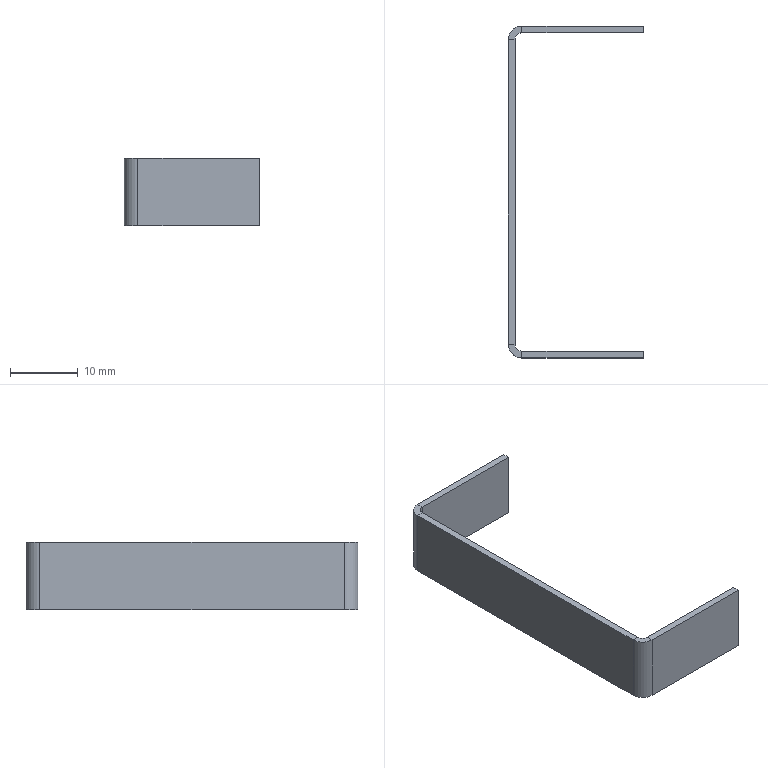Part | SolidWorks | features BaseBody 1 | 1 solid | 22 faces | box 20 x 49 x 10 mm | volume 857.124 mm3 | plane 18 | cylinder 4 | commonest cylinder face diameters 2 x2 4 x2
STEP:
#1=CARTESIAN_POINT('',(20.,48.,0.));
#2=VERTEX_POINT('',#1);
#3=CARTESIAN_POINT('',(2.,48.,0.));
#4=VERTEX_POINT('',#3);
#5=CARTESIAN_POINT('',(0.,48.,0.));
#6=DIRECTION('',(-1.,0.,0.));
#7=VECTOR('',#6,1000.);
#8=LINE('',#5,#7);
#9=EDGE_CURVE('',#2,#4,#8,.T.);
#10=ORIENTED_EDGE('',*,*,#9,.T.);
#11=CARTESIAN_POINT('',(2.,49.,0.));
#12=VERTEX_POINT('',#11);
#13=CARTESIAN_POINT('',(2.,48.,0.));
#14=DIRECTION('',(0.,1.,0.));
#15=VECTOR('',#14,1000.);
#16=LINE('',#13,#15);
#17=EDGE_CURVE('',#4,#12,#16,.T.);
#18=ORIENTED_EDGE('',*,*,#17,.T.);
#19=CARTESIAN_POINT('',(20.,49.,0.));
#20=VERTEX_POINT('',#19);
#21=CARTESIAN_POINT('',(0.,49.,0.));
#22=DIRECTION('',(-1.,0.,0.));
#23=VECTOR('',#22,1000.);
#24=LINE('',#21,#23);
#25=EDGE_CURVE('',#20,#12,#24,.T.);
#26=ORIENTED_EDGE('',*,*,#25,.F.);
#27=CARTESIAN_POINT('',(20.,49.,0.));
#28=DIRECTION('',(0.,-1.,0.));
#29=VECTOR('',#28,1000.);
#30=LINE('',#27,#29);
#31=EDGE_CURVE('',#20,#2,#30,.T.);
#32=ORIENTED_EDGE('',*,*,#31,.T.);
#33=EDGE_LOOP('',(#10,#18,#26,#32));
#34=FACE_OUTER_BOUND('',#33,.T.);
#35=CARTESIAN_POINT('',(2.,2.,0.));
#36=DIRECTION('',(0.,0.,1.));
#37=DIRECTION('',(1.,0.,0.));
#38=AXIS2_PLACEMENT_3D('',#35,#36,#37);
#39=PLANE('',#38);
#40=ADVANCED_FACE('',(#34),#39,.F.);
#41=CARTESIAN_POINT('',(2.,0.,10.));
#42=VERTEX_POINT('',#41);
#43=CARTESIAN_POINT('',(20.,0.,10.));
#44=VERTEX_POINT('',#43);
#45=CARTESIAN_POINT('',(0.,0.,10.));
#46=DIRECTION('',(1.,0.,0.));
#47=VECTOR('',#46,1000.);
#48=LINE('',#45,#47);
#49=EDGE_CURVE('',#42,#44,#48,.T.);
#50=ORIENTED_EDGE('',*,*,#49,.T.);
#51=CARTESIAN_POINT('',(20.,1.,10.));
#52=VERTEX_POINT('',#51);
#53=CARTESIAN_POINT('',(20.,1.,10.));
#54=DIRECTION('',(0.,-1.,0.));
#55=VECTOR('',#54,1000.);
#56=LINE('',#53,#55);
#57=EDGE_CURVE('',#52,#44,#56,.T.);
#58=ORIENTED_EDGE('',*,*,#57,.F.);
#59=CARTESIAN_POINT('',(2.,1.,10.));
#60=VERTEX_POINT('',#59);
#61=CARTESIAN_POINT('',(0.,1.,10.));
#62=DIRECTION('',(1.,0.,0.));
#63=VECTOR('',#62,1000.);
#64=LINE('',#61,#63);
#65=EDGE_CURVE('',#60,#52,#64,.T.);
#66=ORIENTED_EDGE('',*,*,#65,.F.);
#67=CARTESIAN_POINT('',(2.,1.,10.));
#68=DIRECTION('',(0.,-1.,0.));
#69=VECTOR('',#68,1000.);
#70=LINE('',#67,#69);
#71=EDGE_CURVE('',#60,#42,#70,.T.);
#72=ORIENTED_EDGE('',*,*,#71,.T.);
#73=EDGE_LOOP('',(#50,#58,#66,#72));
#74=FACE_OUTER_BOUND('',#73,.T.);
#75=CARTESIAN_POINT('',(2.,2.,10.));
#76=DIRECTION('',(0.,0.,1.));
#77=DIRECTION('',(1.,0.,0.));
#78=AXIS2_PLACEMENT_3D('',#75,#76,#77);
#79=PLANE('',#78);
#80=ADVANCED_FACE('',(#74),#79,.T.);
#81=CARTESIAN_POINT('',(0.,2.,0.));
#82=VERTEX_POINT('',#81);
#83=CARTESIAN_POINT('',(2.,0.,0.));
#84=VERTEX_POINT('',#83);
#85=CARTESIAN_POINT('',(2.,2.,0.));
#86=DIRECTION('',(0.,0.,1.));
#87=DIRECTION('',(-1.,0.,0.));
#88=AXIS2_PLACEMENT_3D('',#85,#86,#87);
#89=CIRCLE('',#88,2.);
#90=EDGE_CURVE('',#82,#84,#89,.T.);
#91=ORIENTED_EDGE('',*,*,#90,.T.);
#92=CARTESIAN_POINT('',(2.,0.,10.));
#93=DIRECTION('',(0.,0.,-1.));
#94=VECTOR('',#93,1000.);
#95=LINE('',#92,#94);
#96=EDGE_CURVE('',#42,#84,#95,.T.);
#97=ORIENTED_EDGE('',*,*,#96,.F.);
#98=CARTESIAN_POINT('',(0.,2.,10.));
#99=VERTEX_POINT('',#98);
#100=CARTESIAN_POINT('',(2.,2.,10.));
#101=DIRECTION('',(0.,0.,1.));
#102=DIRECTION('',(-1.,0.,0.));
#103=AXIS2_PLACEMENT_3D('',#100,#101,#102);
#104=CIRCLE('',#103,2.);
#105=EDGE_CURVE('',#99,#42,#104,.T.);
#106=ORIENTED_EDGE('',*,*,#105,.F.);
#107=CARTESIAN_POINT('',(0.,2.,10.));
#108=DIRECTION('',(0.,0.,-1.));
#109=VECTOR('',#108,1000.);
#110=LINE('',#107,#109);
#111=EDGE_CURVE('',#99,#82,#110,.T.);
#112=ORIENTED_EDGE('',*,*,#111,.T.);
#113=EDGE_LOOP('',(#91,#97,#106,#112));
#114=FACE_OUTER_BOUND('',#113,.T.);
#115=CARTESIAN_POINT('',(2.,2.,10.));
#116=DIRECTION('',(0.,0.,-1.));
#117=DIRECTION('',(-1.,0.,0.));
#118=AXIS2_PLACEMENT_3D('',#115,#116,#117);
#119=CYLINDRICAL_SURFACE('',#118,2.);
#120=ADVANCED_FACE('',(#114),#119,.T.);
#121=CARTESIAN_POINT('',(0.,47.,0.));
#122=VERTEX_POINT('',#121);
#123=CARTESIAN_POINT('',(0.,0.,0.));
#124=DIRECTION('',(0.,-1.,0.));
#125=VECTOR('',#124,1000.);
#126=LINE('',#123,#125);
#127=EDGE_CURVE('',#122,#82,#126,.T.);
#128=ORIENTED_EDGE('',*,*,#127,.T.);
#129=ORIENTED_EDGE('',*,*,#111,.F.);
#130=CARTESIAN_POINT('',(0.,47.,10.));
#131=VERTEX_POINT('',#130);
#132=CARTESIAN_POINT('',(0.,0.,10.));
#133=DIRECTION('',(0.,-1.,0.));
#134=VECTOR('',#133,1000.);
#135=LINE('',#132,#134);
#136=EDGE_CURVE('',#131,#99,#135,.T.);
#137=ORIENTED_EDGE('',*,*,#136,.F.);
#138=CARTESIAN_POINT('',(0.,47.,10.));
#139=DIRECTION('',(0.,0.,-1.));
#140=VECTOR('',#139,1000.);
#141=LINE('',#138,#140);
#142=EDGE_CURVE('',#131,#122,#141,.T.);
#143=ORIENTED_EDGE('',*,*,#142,.T.);
#144=EDGE_LOOP('',(#128,#129,#137,#143));
#145=FACE_OUTER_BOUND('',#144,.T.);
#146=CARTESIAN_POINT('',(0.,0.,10.));
#147=DIRECTION('',(1.,0.,0.));
#148=DIRECTION('',(0.,1.,0.));
#149=AXIS2_PLACEMENT_3D('',#146,#147,#148);
#150=PLANE('',#149);
#151=ADVANCED_FACE('',(#145),#150,.F.);
#152=CARTESIAN_POINT('',(2.,47.,0.));
#153=DIRECTION('',(0.,0.,1.));
#154=DIRECTION('',(-1.,0.,0.));
#155=AXIS2_PLACEMENT_3D('',#152,#153,#154);
#156=CIRCLE('',#155,2.);
#157=EDGE_CURVE('',#12,#122,#156,.T.);
#158=ORIENTED_EDGE('',*,*,#157,.T.);
#159=ORIENTED_EDGE('',*,*,#142,.F.);
#160=CARTESIAN_POINT('',(2.,49.,10.));
#161=VERTEX_POINT('',#160);
#162=CARTESIAN_POINT('',(2.,47.,10.));
#163=DIRECTION('',(0.,0.,1.));
#164=DIRECTION('',(-1.,0.,0.));
#165=AXIS2_PLACEMENT_3D('',#162,#163,#164);
#166=CIRCLE('',#165,2.);
#167=EDGE_CURVE('',#161,#131,#166,.T.);
#168=ORIENTED_EDGE('',*,*,#167,.F.);
#169=CARTESIAN_POINT('',(2.,49.,10.));
#170=DIRECTION('',(0.,0.,-1.));
#171=VECTOR('',#170,1000.);
#172=LINE('',#169,#171);
#173=EDGE_CURVE('',#161,#12,#172,.T.);
#174=ORIENTED_EDGE('',*,*,#173,.T.);
#175=EDGE_LOOP('',(#158,#159,#168,#174));
#176=FACE_OUTER_BOUND('',#175,.T.);
#177=CARTESIAN_POINT('',(2.,47.,10.));
#178=DIRECTION('',(0.,0.,-1.));
#179=DIRECTION('',(-1.,0.,0.));
#180=AXIS2_PLACEMENT_3D('',#177,#178,#179);
#181=CYLINDRICAL_SURFACE('',#180,2.);
#182=ADVANCED_FACE('',(#176),#181,.T.);
#183=ORIENTED_EDGE('',*,*,#25,.T.);
#184=ORIENTED_EDGE('',*,*,#173,.F.);
#185=CARTESIAN_POINT('',(20.,49.,10.));
#186=VERTEX_POINT('',#185);
#187=CARTESIAN_POINT('',(0.,49.,10.));
#188=DIRECTION('',(-1.,0.,0.));
#189=VECTOR('',#188,1000.);
#190=LINE('',#187,#189);
#191=EDGE_CURVE('',#186,#161,#190,.T.);
#192=ORIENTED_EDGE('',*,*,#191,.F.);
#193=CARTESIAN_POINT('',(20.,49.,10.));
#194=DIRECTION('',(0.,0.,-1.));
#195=VECTOR('',#194,1000.);
#196=LINE('',#193,#195);
#197=EDGE_CURVE('',#186,#20,#196,.T.);
#198=ORIENTED_EDGE('',*,*,#197,.T.);
#199=EDGE_LOOP('',(#183,#184,#192,#198));
#200=FACE_OUTER_BOUND('',#199,.T.);
#201=CARTESIAN_POINT('',(0.,49.,10.));
#202=DIRECTION('',(0.,-1.,0.));
#203=DIRECTION('',(0.,0.,-1.));
#204=AXIS2_PLACEMENT_3D('',#201,#202,#203);
#205=PLANE('',#204);
#206=ADVANCED_FACE('',(#200),#205,.F.);
#207=ORIENTED_EDGE('',*,*,#31,.F.);
#208=ORIENTED_EDGE('',*,*,#197,.F.);
#209=CARTESIAN_POINT('',(20.,48.,10.));
#210=VERTEX_POINT('',#209);
#211=CARTESIAN_POINT('',(20.,49.,10.));
#212=DIRECTION('',(0.,-1.,0.));
#213=VECTOR('',#212,1000.);
#214=LINE('',#211,#213);
#215=EDGE_CURVE('',#186,#210,#214,.T.);
#216=ORIENTED_EDGE('',*,*,#215,.T.);
#217=CARTESIAN_POINT('',(20.,48.,10.));
#218=DIRECTION('',(0.,0.,-1.));
#219=VECTOR('',#218,1000.);
#220=LINE('',#217,#219);
#221=EDGE_CURVE('',#210,#2,#220,.T.);
#222=ORIENTED_EDGE('',*,*,#221,.T.);
#223=EDGE_LOOP('',(#207,#208,#216,#222));
#224=FACE_OUTER_BOUND('',#223,.T.);
#225=CARTESIAN_POINT('',(20.,49.,10.));
#226=DIRECTION('',(1.,0.,0.));
#227=DIRECTION('',(0.,1.,0.));
#228=AXIS2_PLACEMENT_3D('',#225,#226,#227);
#229=PLANE('',#228);
#230=ADVANCED_FACE('',(#224),#229,.T.);
#231=ORIENTED_EDGE('',*,*,#9,.F.);
#232=ORIENTED_EDGE('',*,*,#221,.F.);
#233=CARTESIAN_POINT('',(2.,48.,10.));
#234=VERTEX_POINT('',#233);
#235=CARTESIAN_POINT('',(0.,48.,10.));
#236=DIRECTION('',(-1.,0.,0.));
#237=VECTOR('',#236,1000.);
#238=LINE('',#235,#237);
#239=EDGE_CURVE('',#210,#234,#238,.T.);
#240=ORIENTED_EDGE('',*,*,#239,.T.);
#241=CARTESIAN_POINT('',(2.,48.,10.));
#242=DIRECTION('',(0.,0.,-1.));
#243=VECTOR('',#242,1000.);
#244=LINE('',#241,#243);
#245=EDGE_CURVE('',#234,#4,#244,.T.);
#246=ORIENTED_EDGE('',*,*,#245,.T.);
#247=EDGE_LOOP('',(#231,#232,#240,#246));
#248=FACE_OUTER_BOUND('',#247,.T.);
#249=CARTESIAN_POINT('',(0.,48.,10.));
#250=DIRECTION('',(0.,-1.,0.));
#251=DIRECTION('',(0.,0.,-1.));
#252=AXIS2_PLACEMENT_3D('',#249,#250,#251);
#253=PLANE('',#252);
#254=ADVANCED_FACE('',(#248),#253,.T.);
#255=CARTESIAN_POINT('',(1.,47.,0.));
#256=VERTEX_POINT('',#255);
#257=CARTESIAN_POINT('',(2.,47.,0.));
#258=DIRECTION('',(0.,0.,1.));
#259=DIRECTION('',(1.,0.,0.));
#260=AXIS2_PLACEMENT_3D('',#257,#258,#259);
#261=CIRCLE('',#260,1.);
#262=EDGE_CURVE('',#4,#256,#261,.T.);
#263=ORIENTED_EDGE('',*,*,#262,.F.);
#264=ORIENTED_EDGE('',*,*,#245,.F.);
#265=CARTESIAN_POINT('',(1.,47.,10.));
#266=VERTEX_POINT('',#265);
#267=CARTESIAN_POINT('',(2.,47.,10.));
#268=DIRECTION('',(0.,0.,1.));
#269=DIRECTION('',(1.,0.,0.));
#270=AXIS2_PLACEMENT_3D('',#267,#268,#269);
#271=CIRCLE('',#270,1.);
#272=EDGE_CURVE('',#234,#266,#271,.T.);
#273=ORIENTED_EDGE('',*,*,#272,.T.);
#274=CARTESIAN_POINT('',(1.,47.,10.));
#275=DIRECTION('',(0.,0.,-1.));
#276=VECTOR('',#275,1000.);
#277=LINE('',#274,#276);
#278=EDGE_CURVE('',#266,#256,#277,.T.);
#279=ORIENTED_EDGE('',*,*,#278,.T.);
#280=EDGE_LOOP('',(#263,#264,#273,#279));
#281=FACE_OUTER_BOUND('',#280,.T.);
#282=CARTESIAN_POINT('',(2.,47.,10.));
#283=DIRECTION('',(0.,0.,-1.));
#284=DIRECTION('',(-1.,0.,0.));
#285=AXIS2_PLACEMENT_3D('',#282,#283,#284);
#286=CYLINDRICAL_SURFACE('',#285,1.);
#287=ADVANCED_FACE('',(#281),#286,.F.);
#288=CARTESIAN_POINT('',(1.,2.,0.));
#289=VERTEX_POINT('',#288);
#290=CARTESIAN_POINT('',(1.,0.,0.));
#291=DIRECTION('',(0.,-1.,0.));
#292=VECTOR('',#291,1000.);
#293=LINE('',#290,#292);
#294=EDGE_CURVE('',#256,#289,#293,.T.);
#295=ORIENTED_EDGE('',*,*,#294,.F.);
#296=ORIENTED_EDGE('',*,*,#278,.F.);
#297=CARTESIAN_POINT('',(1.,2.,10.));
#298=VERTEX_POINT('',#297);
#299=CARTESIAN_POINT('',(1.,0.,10.));
#300=DIRECTION('',(0.,-1.,0.));
#301=VECTOR('',#300,1000.);
#302=LINE('',#299,#301);
#303=EDGE_CURVE('',#266,#298,#302,.T.);
#304=ORIENTED_EDGE('',*,*,#303,.T.);
#305=CARTESIAN_POINT('',(1.,2.,10.));
#306=DIRECTION('',(0.,0.,-1.));
#307=VECTOR('',#306,1000.);
#308=LINE('',#305,#307);
#309=EDGE_CURVE('',#298,#289,#308,.T.);
#310=ORIENTED_EDGE('',*,*,#309,.T.);
#311=EDGE_LOOP('',(#295,#296,#304,#310));
#312=FACE_OUTER_BOUND('',#311,.T.);
#313=CARTESIAN_POINT('',(1.,0.,10.));
#314=DIRECTION('',(1.,0.,0.));
#315=DIRECTION('',(0.,1.,0.));
#316=AXIS2_PLACEMENT_3D('',#313,#314,#315);
#317=PLANE('',#316);
#318=ADVANCED_FACE('',(#312),#317,.T.);
#319=CARTESIAN_POINT('',(2.,1.,0.));
#320=VERTEX_POINT('',#319);
#321=CARTESIAN_POINT('',(2.,2.,0.));
#322=DIRECTION('',(0.,0.,1.));
#323=DIRECTION('',(1.,0.,0.));
#324=AXIS2_PLACEMENT_3D('',#321,#322,#323);
#325=CIRCLE('',#324,1.);
#326=EDGE_CURVE('',#289,#320,#325,.T.);
#327=ORIENTED_EDGE('',*,*,#326,.F.);
#328=ORIENTED_EDGE('',*,*,#309,.F.);
#329=CARTESIAN_POINT('',(2.,2.,10.));
#330=DIRECTION('',(0.,0.,1.));
#331=DIRECTION('',(1.,0.,0.));
#332=AXIS2_PLACEMENT_3D('',#329,#330,#331);
#333=CIRCLE('',#332,1.);
#334=EDGE_CURVE('',#298,#60,#333,.T.);
#335=ORIENTED_EDGE('',*,*,#334,.T.);
#336=CARTESIAN_POINT('',(2.,1.,10.));
#337=DIRECTION('',(0.,0.,-1.));
#338=VECTOR('',#337,1000.);
#339=LINE('',#336,#338);
#340=EDGE_CURVE('',#60,#320,#339,.T.);
#341=ORIENTED_EDGE('',*,*,#340,.T.);
#342=EDGE_LOOP('',(#327,#328,#335,#341));
#343=FACE_OUTER_BOUND('',#342,.T.);
#344=CARTESIAN_POINT('',(2.,2.,10.));
#345=DIRECTION('',(0.,0.,-1.));
#346=DIRECTION('',(-1.,0.,0.));
#347=AXIS2_PLACEMENT_3D('',#344,#345,#346);
#348=CYLINDRICAL_SURFACE('',#347,1.);
#349=ADVANCED_FACE('',(#343),#348,.F.);
#350=CARTESIAN_POINT('',(20.,1.,0.));
#351=VERTEX_POINT('',#350);
#352=CARTESIAN_POINT('',(0.,1.,0.));
#353=DIRECTION('',(1.,0.,0.));
#354=VECTOR('',#353,1000.);
#355=LINE('',#352,#354);
#356=EDGE_CURVE('',#320,#351,#355,.T.);
#357=ORIENTED_EDGE('',*,*,#356,.F.);
#358=ORIENTED_EDGE('',*,*,#340,.F.);
#359=ORIENTED_EDGE('',*,*,#65,.T.);
#360=CARTESIAN_POINT('',(20.,1.,10.));
#361=DIRECTION('',(0.,0.,-1.));
#362=VECTOR('',#361,1000.);
#363=LINE('',#360,#362);
#364=EDGE_CURVE('',#52,#351,#363,.T.);
#365=ORIENTED_EDGE('',*,*,#364,.T.);
#366=EDGE_LOOP('',(#357,#358,#359,#365));
#367=FACE_OUTER_BOUND('',#366,.T.);
#368=CARTESIAN_POINT('',(0.,1.,10.));
#369=DIRECTION('',(0.,1.,0.));
#370=DIRECTION('',(1.,0.,0.));
#371=AXIS2_PLACEMENT_3D('',#368,#369,#370);
#372=PLANE('',#371);
#373=ADVANCED_FACE('',(#367),#372,.T.);
#374=CARTESIAN_POINT('',(20.,0.,0.));
#375=VERTEX_POINT('',#374);
#376=CARTESIAN_POINT('',(20.,1.,0.));
#377=DIRECTION('',(0.,-1.,0.));
#378=VECTOR('',#377,1000.);
#379=LINE('',#376,#378);
#380=EDGE_CURVE('',#351,#375,#379,.T.);
#381=ORIENTED_EDGE('',*,*,#380,.F.);
#382=ORIENTED_EDGE('',*,*,#364,.F.);
#383=ORIENTED_EDGE('',*,*,#57,.T.);
#384=CARTESIAN_POINT('',(20.,0.,10.));
#385=DIRECTION('',(0.,0.,-1.));
#386=VECTOR('',#385,1000.);
#387=LINE('',#384,#386);
#388=EDGE_CURVE('',#44,#375,#387,.T.);
#389=ORIENTED_EDGE('',*,*,#388,.T.);
#390=EDGE_LOOP('',(#381,#382,#383,#389));
#391=FACE_OUTER_BOUND('',#390,.T.);
#392=CARTESIAN_POINT('',(20.,1.,10.));
#393=DIRECTION('',(1.,0.,0.));
#394=DIRECTION('',(0.,1.,0.));
#395=AXIS2_PLACEMENT_3D('',#392,#393,#394);
#396=PLANE('',#395);
#397=ADVANCED_FACE('',(#391),#396,.T.);
#398=CARTESIAN_POINT('',(0.,0.,0.));
#399=DIRECTION('',(1.,0.,0.));
#400=VECTOR('',#399,1000.);
#401=LINE('',#398,#400);
#402=EDGE_CURVE('',#84,#375,#401,.T.);
#403=ORIENTED_EDGE('',*,*,#402,.T.);
#404=ORIENTED_EDGE('',*,*,#388,.F.);
#405=ORIENTED_EDGE('',*,*,#49,.F.);
#406=ORIENTED_EDGE('',*,*,#96,.T.);
#407=EDGE_LOOP('',(#403,#404,#405,#406));
#408=FACE_OUTER_BOUND('',#407,.T.);
#409=CARTESIAN_POINT('',(0.,0.,10.));
#410=DIRECTION('',(0.,1.,0.));
#411=DIRECTION('',(1.,0.,0.));
#412=AXIS2_PLACEMENT_3D('',#409,#410,#411);
#413=PLANE('',#412);
#414=ADVANCED_FACE('',(#408),#413,.F.);
#415=ORIENTED_EDGE('',*,*,#402,.F.);
#416=CARTESIAN_POINT('',(2.,0.,0.));
#417=DIRECTION('',(0.,1.,0.));
#418=VECTOR('',#417,1000.);
#419=LINE('',#416,#418);
#420=EDGE_CURVE('',#84,#320,#419,.T.);
#421=ORIENTED_EDGE('',*,*,#420,.T.);
#422=ORIENTED_EDGE('',*,*,#356,.T.);
#423=ORIENTED_EDGE('',*,*,#380,.T.);
#424=EDGE_LOOP('',(#415,#421,#422,#423));
#425=FACE_OUTER_BOUND('',#424,.T.);
#426=CARTESIAN_POINT('',(1.,2.,0.));
#427=DIRECTION('',(0.,0.,-1.));
#428=DIRECTION('',(0.,-1.,0.));
#429=AXIS2_PLACEMENT_3D('',#426,#427,#428);
#430=PLANE('',#429);
#431=ADVANCED_FACE('',(#425),#430,.T.);
#432=ORIENTED_EDGE('',*,*,#420,.F.);
#433=ORIENTED_EDGE('',*,*,#90,.F.);
#434=CARTESIAN_POINT('',(1.,2.,0.));
#435=DIRECTION('',(-1.,0.,0.));
#436=VECTOR('',#435,1000.);
#437=LINE('',#434,#436);
#438=EDGE_CURVE('',#289,#82,#437,.T.);
#439=ORIENTED_EDGE('',*,*,#438,.F.);
#440=ORIENTED_EDGE('',*,*,#326,.T.);
#441=EDGE_LOOP('',(#432,#433,#439,#440));
#442=FACE_OUTER_BOUND('',#441,.T.);
#443=CARTESIAN_POINT('',(2.,0.,0.));
#444=DIRECTION('',(0.,0.,-1.));
#445=DIRECTION('',(0.,-1.,0.));
#446=AXIS2_PLACEMENT_3D('',#443,#444,#445);
#447=PLANE('',#446);
#448=ADVANCED_FACE('',(#442),#447,.T.);
#449=ORIENTED_EDGE('',*,*,#136,.T.);
#450=CARTESIAN_POINT('',(0.,2.,10.));
#451=DIRECTION('',(1.,0.,0.));
#452=VECTOR('',#451,1000.);
#453=LINE('',#450,#452);
#454=EDGE_CURVE('',#99,#298,#453,.T.);
#455=ORIENTED_EDGE('',*,*,#454,.T.);
#456=ORIENTED_EDGE('',*,*,#303,.F.);
#457=CARTESIAN_POINT('',(1.,47.,10.));
#458=DIRECTION('',(-1.,0.,0.));
#459=VECTOR('',#458,1000.);
#460=LINE('',#457,#459);
#461=EDGE_CURVE('',#266,#131,#460,.T.);
#462=ORIENTED_EDGE('',*,*,#461,.T.);
#463=EDGE_LOOP('',(#449,#455,#456,#462));
#464=FACE_OUTER_BOUND('',#463,.T.);
#465=CARTESIAN_POINT('',(2.,1.,10.));
#466=DIRECTION('',(0.,0.,1.));
#467=DIRECTION('',(1.,0.,0.));
#468=AXIS2_PLACEMENT_3D('',#465,#466,#467);
#469=PLANE('',#468);
#470=ADVANCED_FACE('',(#464),#469,.T.);
#471=ORIENTED_EDGE('',*,*,#454,.F.);
#472=ORIENTED_EDGE('',*,*,#105,.T.);
#473=ORIENTED_EDGE('',*,*,#71,.F.);
#474=ORIENTED_EDGE('',*,*,#334,.F.);
#475=EDGE_LOOP('',(#471,#472,#473,#474));
#476=FACE_OUTER_BOUND('',#475,.T.);
#477=CARTESIAN_POINT('',(0.,2.,10.));
#478=DIRECTION('',(0.,0.,1.));
#479=DIRECTION('',(1.,0.,0.));
#480=AXIS2_PLACEMENT_3D('',#477,#478,#479);
#481=PLANE('',#480);
#482=ADVANCED_FACE('',(#476),#481,.T.);
#483=ORIENTED_EDGE('',*,*,#127,.F.);
#484=CARTESIAN_POINT('',(0.,47.,0.));
#485=DIRECTION('',(1.,0.,0.));
#486=VECTOR('',#485,1000.);
#487=LINE('',#484,#486);
#488=EDGE_CURVE('',#122,#256,#487,.T.);
#489=ORIENTED_EDGE('',*,*,#488,.T.);
#490=ORIENTED_EDGE('',*,*,#294,.T.);
#491=ORIENTED_EDGE('',*,*,#438,.T.);
#492=EDGE_LOOP('',(#483,#489,#490,#491));
#493=FACE_OUTER_BOUND('',#492,.T.);
#494=CARTESIAN_POINT('',(2.,48.,0.));
#495=DIRECTION('',(0.,0.,-1.));
#496=DIRECTION('',(0.,-1.,0.));
#497=AXIS2_PLACEMENT_3D('',#494,#495,#496);
#498=PLANE('',#497);
#499=ADVANCED_FACE('',(#493),#498,.T.);
#500=ORIENTED_EDGE('',*,*,#488,.F.);
#501=ORIENTED_EDGE('',*,*,#157,.F.);
#502=ORIENTED_EDGE('',*,*,#17,.F.);
#503=ORIENTED_EDGE('',*,*,#262,.T.);
#504=EDGE_LOOP('',(#500,#501,#502,#503));
#505=FACE_OUTER_BOUND('',#504,.T.);
#506=CARTESIAN_POINT('',(0.,47.,0.));
#507=DIRECTION('',(0.,0.,-1.));
#508=DIRECTION('',(0.,-1.,0.));
#509=AXIS2_PLACEMENT_3D('',#506,#507,#508);
#510=PLANE('',#509);
#511=ADVANCED_FACE('',(#505),#510,.T.);
#512=ORIENTED_EDGE('',*,*,#191,.T.);
#513=CARTESIAN_POINT('',(2.,49.,10.));
#514=DIRECTION('',(0.,-1.,0.));
#515=VECTOR('',#514,1000.);
#516=LINE('',#513,#515);
#517=EDGE_CURVE('',#161,#234,#516,.T.);
#518=ORIENTED_EDGE('',*,*,#517,.T.);
#519=ORIENTED_EDGE('',*,*,#239,.F.);
#520=ORIENTED_EDGE('',*,*,#215,.F.);
#521=EDGE_LOOP('',(#512,#518,#519,#520));
#522=FACE_OUTER_BOUND('',#521,.T.);
#523=CARTESIAN_POINT('',(1.,47.,10.));
#524=DIRECTION('',(0.,0.,1.));
#525=DIRECTION('',(1.,0.,0.));
#526=AXIS2_PLACEMENT_3D('',#523,#524,#525);
#527=PLANE('',#526);
#528=ADVANCED_FACE('',(#522),#527,.T.);
#529=ORIENTED_EDGE('',*,*,#517,.F.);
#530=ORIENTED_EDGE('',*,*,#167,.T.);
#531=ORIENTED_EDGE('',*,*,#461,.F.);
#532=ORIENTED_EDGE('',*,*,#272,.F.);
#533=EDGE_LOOP('',(#529,#530,#531,#532));
#534=FACE_OUTER_BOUND('',#533,.T.);
#535=CARTESIAN_POINT('',(2.,49.,10.));
#536=DIRECTION('',(0.,0.,1.));
#537=DIRECTION('',(1.,0.,0.));
#538=AXIS2_PLACEMENT_3D('',#535,#536,#537);
#539=PLANE('',#538);
#540=ADVANCED_FACE('',(#534),#539,.T.);
#541=CLOSED_SHELL('',(#40,#80,#120,#151,#182,#206,#230,#254,#287,#318,#349,#373,#397,#414,#431,#448,#470,#482,#499,#511,#528,#540));
#542=MANIFOLD_SOLID_BREP('',#541);
#543=CARTESIAN_POINT('',(0.,0.,0.));
#544=DIRECTION('',(0.,0.,1.));
#545=DIRECTION('',(1.,0.,0.));
#546=AXIS2_PLACEMENT_3D('',#543,#544,#545);
#547=(LENGTH_UNIT()NAMED_UNIT(*)SI_UNIT(.MILLI.,.METRE.));
#548=UNCERTAINTY_MEASURE_WITH_UNIT(LENGTH_MEASURE(0.00001),#547,'','');
#549=(NAMED_UNIT(*)PLANE_ANGLE_UNIT()SI_UNIT($,.RADIAN.));
#550=(NAMED_UNIT(*)SI_UNIT($,.STERADIAN.)SOLID_ANGLE_UNIT());
#551=(GEOMETRIC_REPRESENTATION_CONTEXT(3)GLOBAL_UNCERTAINTY_ASSIGNED_CONTEXT((#548))GLOBAL_UNIT_ASSIGNED_CONTEXT((#547,#549,#550))REPRESENTATION_CONTEXT('',''));
#552=ADVANCED_BREP_SHAPE_REPRESENTATION('',(#542,#546),#551);